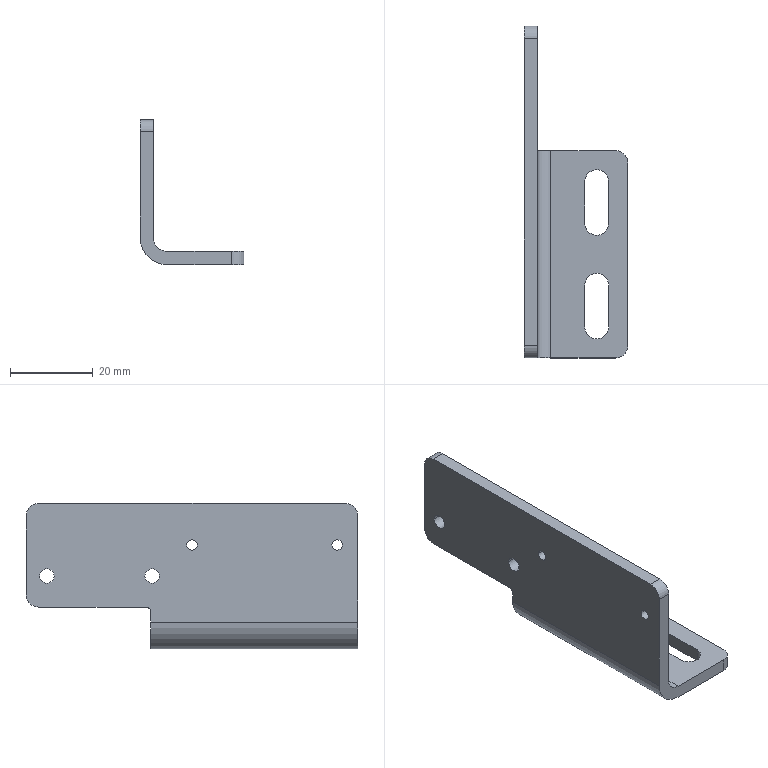Part | STEP file | J014-EBZ05-06-06-Part-1 | 1 solid | 34 faces | box 25 x 80 x 35 mm | volume 10495 mm3 | cylinder 20 | plane 14 | commonest cylinder face diameters 6 x5 2.5 x4 3.5 x4 5.8 x4 2 x1 6.4 x1
STEP:
#1=CARTESIAN_POINT('',(0.,3.75,25.));
#2=VERTEX_POINT('',#1);
#3=CARTESIAN_POINT('',(0.,6.25,25.));
#4=VERTEX_POINT('',#3);
#5=CARTESIAN_POINT('',(0.,5.,25.));
#6=DIRECTION('',(1.,0.,0.));
#7=DIRECTION('',(0.,1.,0.));
#8=AXIS2_PLACEMENT_3D('',#5,#6,#7);
#9=CIRCLE('',#8,1.25);
#10=EDGE_CURVE('',#2,#4,#9,.T.);
#11=ORIENTED_EDGE('',*,*,#10,.F.);
#12=CARTESIAN_POINT('',(3.2,3.75,25.));
#13=VERTEX_POINT('',#12);
#14=CARTESIAN_POINT('',(0.,3.75,25.));
#15=DIRECTION('',(1.,0.,0.));
#16=VECTOR('',#15,1000.);
#17=LINE('',#14,#16);
#18=EDGE_CURVE('',#2,#13,#17,.T.);
#19=ORIENTED_EDGE('',*,*,#18,.T.);
#20=CARTESIAN_POINT('',(3.2,6.25,25.));
#21=VERTEX_POINT('',#20);
#22=CARTESIAN_POINT('',(3.2,5.,25.));
#23=DIRECTION('',(-1.,0.,0.));
#24=DIRECTION('',(0.,-1.,0.));
#25=AXIS2_PLACEMENT_3D('',#22,#23,#24);
#26=CIRCLE('',#25,1.25);
#27=EDGE_CURVE('',#21,#13,#26,.T.);
#28=ORIENTED_EDGE('',*,*,#27,.F.);
#29=CARTESIAN_POINT('',(0.,6.25,25.));
#30=DIRECTION('',(1.,0.,0.));
#31=VECTOR('',#30,1000.);
#32=LINE('',#29,#31);
#33=EDGE_CURVE('',#4,#21,#32,.T.);
#34=ORIENTED_EDGE('',*,*,#33,.F.);
#35=EDGE_LOOP('',(#11,#19,#28,#34));
#36=FACE_OUTER_BOUND('',#35,.T.);
#37=CARTESIAN_POINT('',(0.,5.,25.));
#38=DIRECTION('',(1.,0.,0.));
#39=DIRECTION('',(0.,1.,0.));
#40=AXIS2_PLACEMENT_3D('',#37,#38,#39);
#41=CYLINDRICAL_SURFACE('',#40,1.25);
#42=ADVANCED_FACE('',(#36),#41,.F.);
#43=CARTESIAN_POINT('',(0.,38.75,25.));
#44=VERTEX_POINT('',#43);
#45=CARTESIAN_POINT('',(0.,41.25,25.));
#46=VERTEX_POINT('',#45);
#47=CARTESIAN_POINT('',(0.,40.,25.));
#48=DIRECTION('',(1.,0.,0.));
#49=DIRECTION('',(0.,1.,0.));
#50=AXIS2_PLACEMENT_3D('',#47,#48,#49);
#51=CIRCLE('',#50,1.25);
#52=EDGE_CURVE('',#44,#46,#51,.T.);
#53=ORIENTED_EDGE('',*,*,#52,.F.);
#54=CARTESIAN_POINT('',(3.2,38.75,25.));
#55=VERTEX_POINT('',#54);
#56=CARTESIAN_POINT('',(0.,38.75,25.));
#57=DIRECTION('',(1.,0.,0.));
#58=VECTOR('',#57,1000.);
#59=LINE('',#56,#58);
#60=EDGE_CURVE('',#44,#55,#59,.T.);
#61=ORIENTED_EDGE('',*,*,#60,.T.);
#62=CARTESIAN_POINT('',(3.2,41.25,25.));
#63=VERTEX_POINT('',#62);
#64=CARTESIAN_POINT('',(3.2,40.,25.));
#65=DIRECTION('',(-1.,0.,0.));
#66=DIRECTION('',(0.,-1.,0.));
#67=AXIS2_PLACEMENT_3D('',#64,#65,#66);
#68=CIRCLE('',#67,1.25);
#69=EDGE_CURVE('',#63,#55,#68,.T.);
#70=ORIENTED_EDGE('',*,*,#69,.F.);
#71=CARTESIAN_POINT('',(0.,41.25,25.));
#72=DIRECTION('',(1.,0.,0.));
#73=VECTOR('',#72,1000.);
#74=LINE('',#71,#73);
#75=EDGE_CURVE('',#46,#63,#74,.T.);
#76=ORIENTED_EDGE('',*,*,#75,.F.);
#77=EDGE_LOOP('',(#53,#61,#70,#76));
#78=FACE_OUTER_BOUND('',#77,.T.);
#79=CARTESIAN_POINT('',(0.,40.,25.));
#80=DIRECTION('',(1.,0.,0.));
#81=DIRECTION('',(0.,1.,0.));
#82=AXIS2_PLACEMENT_3D('',#79,#80,#81);
#83=CYLINDRICAL_SURFACE('',#82,1.25);
#84=ADVANCED_FACE('',(#78),#83,.F.);
#85=CARTESIAN_POINT('',(3.2,51.35,17.5));
#86=VERTEX_POINT('',#85);
#87=CARTESIAN_POINT('',(3.2,47.85,17.5));
#88=VERTEX_POINT('',#87);
#89=CARTESIAN_POINT('',(3.2,49.6,17.5));
#90=DIRECTION('',(-1.,0.,0.));
#91=DIRECTION('',(0.,-1.,0.));
#92=AXIS2_PLACEMENT_3D('',#89,#90,#91);
#93=CIRCLE('',#92,1.75);
#94=EDGE_CURVE('',#86,#88,#93,.T.);
#95=ORIENTED_EDGE('',*,*,#94,.F.);
#96=CARTESIAN_POINT('',(0.,51.35,17.5));
#97=VERTEX_POINT('',#96);
#98=CARTESIAN_POINT('',(3.2,51.35,17.5));
#99=DIRECTION('',(-1.,0.,0.));
#100=VECTOR('',#99,1000.);
#101=LINE('',#98,#100);
#102=EDGE_CURVE('',#86,#97,#101,.T.);
#103=ORIENTED_EDGE('',*,*,#102,.T.);
#104=CARTESIAN_POINT('',(0.,47.85,17.5));
#105=VERTEX_POINT('',#104);
#106=CARTESIAN_POINT('',(0.,49.6,17.5));
#107=DIRECTION('',(1.,0.,0.));
#108=DIRECTION('',(0.,1.,0.));
#109=AXIS2_PLACEMENT_3D('',#106,#107,#108);
#110=CIRCLE('',#109,1.75);
#111=EDGE_CURVE('',#105,#97,#110,.T.);
#112=ORIENTED_EDGE('',*,*,#111,.F.);
#113=CARTESIAN_POINT('',(3.2,47.85,17.5));
#114=DIRECTION('',(-1.,0.,0.));
#115=VECTOR('',#114,1000.);
#116=LINE('',#113,#115);
#117=EDGE_CURVE('',#88,#105,#116,.T.);
#118=ORIENTED_EDGE('',*,*,#117,.F.);
#119=EDGE_LOOP('',(#95,#103,#112,#118));
#120=FACE_OUTER_BOUND('',#119,.T.);
#121=CARTESIAN_POINT('',(3.2,49.6,17.5));
#122=DIRECTION('',(-1.,0.,0.));
#123=DIRECTION('',(0.,-1.,0.));
#124=AXIS2_PLACEMENT_3D('',#121,#122,#123);
#125=CYLINDRICAL_SURFACE('',#124,1.75);
#126=ADVANCED_FACE('',(#120),#125,.F.);
#127=CARTESIAN_POINT('',(3.2,76.75,17.5));
#128=VERTEX_POINT('',#127);
#129=CARTESIAN_POINT('',(3.2,73.25,17.5));
#130=VERTEX_POINT('',#129);
#131=CARTESIAN_POINT('',(3.2,75.,17.5));
#132=DIRECTION('',(-1.,0.,0.));
#133=DIRECTION('',(0.,-1.,0.));
#134=AXIS2_PLACEMENT_3D('',#131,#132,#133);
#135=CIRCLE('',#134,1.75);
#136=EDGE_CURVE('',#128,#130,#135,.T.);
#137=ORIENTED_EDGE('',*,*,#136,.F.);
#138=CARTESIAN_POINT('',(0.,76.75,17.5));
#139=VERTEX_POINT('',#138);
#140=CARTESIAN_POINT('',(3.2,76.75,17.5));
#141=DIRECTION('',(-1.,0.,0.));
#142=VECTOR('',#141,1000.);
#143=LINE('',#140,#142);
#144=EDGE_CURVE('',#128,#139,#143,.T.);
#145=ORIENTED_EDGE('',*,*,#144,.T.);
#146=CARTESIAN_POINT('',(0.,73.25,17.5));
#147=VERTEX_POINT('',#146);
#148=CARTESIAN_POINT('',(0.,75.,17.5));
#149=DIRECTION('',(1.,0.,0.));
#150=DIRECTION('',(0.,1.,0.));
#151=AXIS2_PLACEMENT_3D('',#148,#149,#150);
#152=CIRCLE('',#151,1.75);
#153=EDGE_CURVE('',#147,#139,#152,.T.);
#154=ORIENTED_EDGE('',*,*,#153,.F.);
#155=CARTESIAN_POINT('',(3.2,73.25,17.5));
#156=DIRECTION('',(-1.,0.,0.));
#157=VECTOR('',#156,1000.);
#158=LINE('',#155,#157);
#159=EDGE_CURVE('',#130,#147,#158,.T.);
#160=ORIENTED_EDGE('',*,*,#159,.F.);
#161=EDGE_LOOP('',(#137,#145,#154,#160));
#162=FACE_OUTER_BOUND('',#161,.T.);
#163=CARTESIAN_POINT('',(3.2,75.,17.5));
#164=DIRECTION('',(-1.,0.,0.));
#165=DIRECTION('',(0.,-1.,0.));
#166=AXIS2_PLACEMENT_3D('',#163,#164,#165);
#167=CYLINDRICAL_SURFACE('',#166,1.75);
#168=ADVANCED_FACE('',(#162),#167,.F.);
#169=CARTESIAN_POINT('',(25.,47.,3.2));
#170=VERTEX_POINT('',#169);
#171=CARTESIAN_POINT('',(25.,3.,3.2));
#172=VERTEX_POINT('',#171);
#173=CARTESIAN_POINT('',(25.,25.,3.2));
#174=DIRECTION('',(0.,-1.,0.));
#175=VECTOR('',#174,1000.);
#176=LINE('',#173,#175);
#177=EDGE_CURVE('',#170,#172,#176,.T.);
#178=ORIENTED_EDGE('',*,*,#177,.F.);
#179=CARTESIAN_POINT('',(22.,50.,3.2));
#180=VERTEX_POINT('',#179);
#181=CARTESIAN_POINT('',(22.,47.,3.2));
#182=DIRECTION('',(0.,0.,1.));
#183=DIRECTION('',(1.,0.,0.));
#184=AXIS2_PLACEMENT_3D('',#181,#182,#183);
#185=CIRCLE('',#184,3.);
#186=EDGE_CURVE('',#170,#180,#185,.T.);
#187=ORIENTED_EDGE('',*,*,#186,.T.);
#188=CARTESIAN_POINT('',(6.4,50.,3.2));
#189=VERTEX_POINT('',#188);
#190=CARTESIAN_POINT('',(12.5,50.,3.2));
#191=DIRECTION('',(1.,0.,0.));
#192=VECTOR('',#191,1000.);
#193=LINE('',#190,#192);
#194=EDGE_CURVE('',#189,#180,#193,.T.);
#195=ORIENTED_EDGE('',*,*,#194,.F.);
#196=CARTESIAN_POINT('',(6.4,0.,3.2));
#197=VERTEX_POINT('',#196);
#198=CARTESIAN_POINT('',(6.4,0.,3.2));
#199=DIRECTION('',(0.,-1.,0.));
#200=VECTOR('',#199,1000.);
#201=LINE('',#198,#200);
#202=EDGE_CURVE('',#189,#197,#201,.T.);
#203=ORIENTED_EDGE('',*,*,#202,.T.);
#204=CARTESIAN_POINT('',(22.,0.,3.2));
#205=VERTEX_POINT('',#204);
#206=CARTESIAN_POINT('',(12.5,0.,3.2));
#207=DIRECTION('',(-1.,0.,0.));
#208=VECTOR('',#207,1000.);
#209=LINE('',#206,#208);
#210=EDGE_CURVE('',#205,#197,#209,.T.);
#211=ORIENTED_EDGE('',*,*,#210,.F.);
#212=CARTESIAN_POINT('',(22.,3.,3.2));
#213=DIRECTION('',(0.,0.,1.));
#214=DIRECTION('',(1.,0.,0.));
#215=AXIS2_PLACEMENT_3D('',#212,#213,#214);
#216=CIRCLE('',#215,3.);
#217=EDGE_CURVE('',#205,#172,#216,.T.);
#218=ORIENTED_EDGE('',*,*,#217,.T.);
#219=EDGE_LOOP('',(#178,#187,#195,#203,#211,#218));
#220=FACE_OUTER_BOUND('',#219,.T.);
#221=CARTESIAN_POINT('',(14.6,7.5,3.2));
#222=VERTEX_POINT('',#221);
#223=CARTESIAN_POINT('',(14.6,17.5,3.2));
#224=VERTEX_POINT('',#223);
#225=CARTESIAN_POINT('',(14.6,12.5,3.2));
#226=DIRECTION('',(0.,1.,0.));
#227=VECTOR('',#226,1000.);
#228=LINE('',#225,#227);
#229=EDGE_CURVE('',#222,#224,#228,.T.);
#230=ORIENTED_EDGE('',*,*,#229,.T.);
#231=CARTESIAN_POINT('',(20.4,17.5,3.2));
#232=VERTEX_POINT('',#231);
#233=CARTESIAN_POINT('',(17.5,17.5,3.2));
#234=DIRECTION('',(0.,0.,-1.));
#235=DIRECTION('',(-1.,0.,0.));
#236=AXIS2_PLACEMENT_3D('',#233,#234,#235);
#237=CIRCLE('',#236,2.9);
#238=EDGE_CURVE('',#224,#232,#237,.T.);
#239=ORIENTED_EDGE('',*,*,#238,.T.);
#240=CARTESIAN_POINT('',(20.4,7.5,3.2));
#241=VERTEX_POINT('',#240);
#242=CARTESIAN_POINT('',(20.4,12.5,3.2));
#243=DIRECTION('',(0.,-1.,0.));
#244=VECTOR('',#243,1000.);
#245=LINE('',#242,#244);
#246=EDGE_CURVE('',#232,#241,#245,.T.);
#247=ORIENTED_EDGE('',*,*,#246,.T.);
#248=CARTESIAN_POINT('',(17.5,7.5,3.2));
#249=DIRECTION('',(0.,0.,-1.));
#250=DIRECTION('',(-1.,0.,0.));
#251=AXIS2_PLACEMENT_3D('',#248,#249,#250);
#252=CIRCLE('',#251,2.9);
#253=EDGE_CURVE('',#241,#222,#252,.T.);
#254=ORIENTED_EDGE('',*,*,#253,.T.);
#255=EDGE_LOOP('',(#230,#239,#247,#254));
#256=FACE_BOUND('',#255,.T.);
#257=CARTESIAN_POINT('',(14.6,32.5,3.2));
#258=VERTEX_POINT('',#257);
#259=CARTESIAN_POINT('',(14.6,42.5,3.2));
#260=VERTEX_POINT('',#259);
#261=CARTESIAN_POINT('',(14.6,37.5,3.2));
#262=DIRECTION('',(0.,1.,0.));
#263=VECTOR('',#262,1000.);
#264=LINE('',#261,#263);
#265=EDGE_CURVE('',#258,#260,#264,.T.);
#266=ORIENTED_EDGE('',*,*,#265,.T.);
#267=CARTESIAN_POINT('',(20.4,42.5,3.2));
#268=VERTEX_POINT('',#267);
#269=CARTESIAN_POINT('',(17.5,42.5,3.2));
#270=DIRECTION('',(0.,0.,-1.));
#271=DIRECTION('',(-1.,0.,0.));
#272=AXIS2_PLACEMENT_3D('',#269,#270,#271);
#273=CIRCLE('',#272,2.9);
#274=EDGE_CURVE('',#260,#268,#273,.T.);
#275=ORIENTED_EDGE('',*,*,#274,.T.);
#276=CARTESIAN_POINT('',(20.4,32.5,3.2));
#277=VERTEX_POINT('',#276);
#278=CARTESIAN_POINT('',(20.4,37.5,3.2));
#279=DIRECTION('',(0.,-1.,0.));
#280=VECTOR('',#279,1000.);
#281=LINE('',#278,#280);
#282=EDGE_CURVE('',#268,#277,#281,.T.);
#283=ORIENTED_EDGE('',*,*,#282,.T.);
#284=CARTESIAN_POINT('',(17.5,32.5,3.2));
#285=DIRECTION('',(0.,0.,-1.));
#286=DIRECTION('',(-1.,0.,0.));
#287=AXIS2_PLACEMENT_3D('',#284,#285,#286);
#288=CIRCLE('',#287,2.9);
#289=EDGE_CURVE('',#277,#258,#288,.T.);
#290=ORIENTED_EDGE('',*,*,#289,.T.);
#291=EDGE_LOOP('',(#266,#275,#283,#290));
#292=FACE_BOUND('',#291,.T.);
#293=CARTESIAN_POINT('',(12.5,25.,3.2));
#294=DIRECTION('',(0.,0.,1.));
#295=DIRECTION('',(1.,0.,0.));
#296=AXIS2_PLACEMENT_3D('',#293,#294,#295);
#297=PLANE('',#296);
#298=ADVANCED_FACE('',(#220,#256,#292),#297,.T.);
#299=CARTESIAN_POINT('',(22.,50.,0.));
#300=VERTEX_POINT('',#299);
#301=CARTESIAN_POINT('',(6.4,50.,0.));
#302=VERTEX_POINT('',#301);
#303=CARTESIAN_POINT('',(12.5,50.,0.));
#304=DIRECTION('',(-1.,0.,0.));
#305=VECTOR('',#304,1000.);
#306=LINE('',#303,#305);
#307=EDGE_CURVE('',#300,#302,#306,.T.);
#308=ORIENTED_EDGE('',*,*,#307,.F.);
#309=CARTESIAN_POINT('',(25.,47.,0.));
#310=VERTEX_POINT('',#309);
#311=CARTESIAN_POINT('',(22.,47.,0.));
#312=DIRECTION('',(0.,0.,-1.));
#313=DIRECTION('',(-1.,0.,0.));
#314=AXIS2_PLACEMENT_3D('',#311,#312,#313);
#315=CIRCLE('',#314,3.);
#316=EDGE_CURVE('',#300,#310,#315,.T.);
#317=ORIENTED_EDGE('',*,*,#316,.T.);
#318=CARTESIAN_POINT('',(25.,3.,0.));
#319=VERTEX_POINT('',#318);
#320=CARTESIAN_POINT('',(25.,25.,0.));
#321=DIRECTION('',(0.,1.,0.));
#322=VECTOR('',#321,1000.);
#323=LINE('',#320,#322);
#324=EDGE_CURVE('',#319,#310,#323,.T.);
#325=ORIENTED_EDGE('',*,*,#324,.F.);
#326=CARTESIAN_POINT('',(22.,0.,0.));
#327=VERTEX_POINT('',#326);
#328=CARTESIAN_POINT('',(22.,3.,0.));
#329=DIRECTION('',(0.,0.,-1.));
#330=DIRECTION('',(-1.,0.,0.));
#331=AXIS2_PLACEMENT_3D('',#328,#329,#330);
#332=CIRCLE('',#331,3.);
#333=EDGE_CURVE('',#319,#327,#332,.T.);
#334=ORIENTED_EDGE('',*,*,#333,.T.);
#335=CARTESIAN_POINT('',(6.4,0.,0.));
#336=VERTEX_POINT('',#335);
#337=CARTESIAN_POINT('',(12.5,0.,0.));
#338=DIRECTION('',(1.,0.,0.));
#339=VECTOR('',#338,1000.);
#340=LINE('',#337,#339);
#341=EDGE_CURVE('',#336,#327,#340,.T.);
#342=ORIENTED_EDGE('',*,*,#341,.F.);
#343=CARTESIAN_POINT('',(6.4,25.,0.));
#344=DIRECTION('',(0.,1.,0.));
#345=VECTOR('',#344,1000.);
#346=LINE('',#343,#345);
#347=EDGE_CURVE('',#336,#302,#346,.T.);
#348=ORIENTED_EDGE('',*,*,#347,.T.);
#349=EDGE_LOOP('',(#308,#317,#325,#334,#342,#348));
#350=FACE_OUTER_BOUND('',#349,.T.);
#351=CARTESIAN_POINT('',(20.4,7.5,0.));
#352=VERTEX_POINT('',#351);
#353=CARTESIAN_POINT('',(20.4,17.5,0.));
#354=VERTEX_POINT('',#353);
#355=CARTESIAN_POINT('',(20.4,12.5,0.));
#356=DIRECTION('',(0.,1.,0.));
#357=VECTOR('',#356,1000.);
#358=LINE('',#355,#357);
#359=EDGE_CURVE('',#352,#354,#358,.T.);
#360=ORIENTED_EDGE('',*,*,#359,.T.);
#361=CARTESIAN_POINT('',(14.6,17.5,0.));
#362=VERTEX_POINT('',#361);
#363=CARTESIAN_POINT('',(17.5,17.5,0.));
#364=DIRECTION('',(0.,0.,1.));
#365=DIRECTION('',(1.,0.,0.));
#366=AXIS2_PLACEMENT_3D('',#363,#364,#365);
#367=CIRCLE('',#366,2.9);
#368=EDGE_CURVE('',#354,#362,#367,.T.);
#369=ORIENTED_EDGE('',*,*,#368,.T.);
#370=CARTESIAN_POINT('',(14.6,7.5,0.));
#371=VERTEX_POINT('',#370);
#372=CARTESIAN_POINT('',(14.6,12.5,0.));
#373=DIRECTION('',(0.,-1.,0.));
#374=VECTOR('',#373,1000.);
#375=LINE('',#372,#374);
#376=EDGE_CURVE('',#362,#371,#375,.T.);
#377=ORIENTED_EDGE('',*,*,#376,.T.);
#378=CARTESIAN_POINT('',(17.5,7.5,0.));
#379=DIRECTION('',(0.,0.,1.));
#380=DIRECTION('',(1.,0.,0.));
#381=AXIS2_PLACEMENT_3D('',#378,#379,#380);
#382=CIRCLE('',#381,2.9);
#383=EDGE_CURVE('',#371,#352,#382,.T.);
#384=ORIENTED_EDGE('',*,*,#383,.T.);
#385=EDGE_LOOP('',(#360,#369,#377,#384));
#386=FACE_BOUND('',#385,.T.);
#387=CARTESIAN_POINT('',(20.4,32.5,0.));
#388=VERTEX_POINT('',#387);
#389=CARTESIAN_POINT('',(20.4,42.5,0.));
#390=VERTEX_POINT('',#389);
#391=CARTESIAN_POINT('',(20.4,37.5,0.));
#392=DIRECTION('',(0.,1.,0.));
#393=VECTOR('',#392,1000.);
#394=LINE('',#391,#393);
#395=EDGE_CURVE('',#388,#390,#394,.T.);
#396=ORIENTED_EDGE('',*,*,#395,.T.);
#397=CARTESIAN_POINT('',(14.6,42.5,0.));
#398=VERTEX_POINT('',#397);
#399=CARTESIAN_POINT('',(17.5,42.5,0.));
#400=DIRECTION('',(0.,0.,1.));
#401=DIRECTION('',(1.,0.,0.));
#402=AXIS2_PLACEMENT_3D('',#399,#400,#401);
#403=CIRCLE('',#402,2.9);
#404=EDGE_CURVE('',#390,#398,#403,.T.);
#405=ORIENTED_EDGE('',*,*,#404,.T.);
#406=CARTESIAN_POINT('',(14.6,32.5,0.));
#407=VERTEX_POINT('',#406);
#408=CARTESIAN_POINT('',(14.6,37.5,0.));
#409=DIRECTION('',(0.,-1.,0.));
#410=VECTOR('',#409,1000.);
#411=LINE('',#408,#410);
#412=EDGE_CURVE('',#398,#407,#411,.T.);
#413=ORIENTED_EDGE('',*,*,#412,.T.);
#414=CARTESIAN_POINT('',(17.5,32.5,0.));
#415=DIRECTION('',(0.,0.,1.));
#416=DIRECTION('',(1.,0.,0.));
#417=AXIS2_PLACEMENT_3D('',#414,#415,#416);
#418=CIRCLE('',#417,2.9);
#419=EDGE_CURVE('',#407,#388,#418,.T.);
#420=ORIENTED_EDGE('',*,*,#419,.T.);
#421=EDGE_LOOP('',(#396,#405,#413,#420));
#422=FACE_BOUND('',#421,.T.);
#423=CARTESIAN_POINT('',(12.5,25.,0.));
#424=DIRECTION('',(0.,0.,-1.));
#425=DIRECTION('',(-1.,0.,0.));
#426=AXIS2_PLACEMENT_3D('',#423,#424,#425);
#427=PLANE('',#426);
#428=ADVANCED_FACE('',(#350,#386,#422),#427,.T.);
#429=CARTESIAN_POINT('',(3.2,0.,6.4));
#430=VERTEX_POINT('',#429);
#431=CARTESIAN_POINT('',(3.2,0.,32.));
#432=VERTEX_POINT('',#431);
#433=CARTESIAN_POINT('',(3.2,0.,5.));
#434=DIRECTION('',(0.,0.,1.));
#435=VECTOR('',#434,1000.);
#436=LINE('',#433,#435);
#437=EDGE_CURVE('',#430,#432,#436,.T.);
#438=ORIENTED_EDGE('',*,*,#437,.T.);
#439=CARTESIAN_POINT('',(0.,0.,32.));
#440=VERTEX_POINT('',#439);
#441=CARTESIAN_POINT('',(12.5,0.,32.));
#442=DIRECTION('',(-1.,0.,0.));
#443=VECTOR('',#442,1000.);
#444=LINE('',#441,#443);
#445=EDGE_CURVE('',#432,#440,#444,.T.);
#446=ORIENTED_EDGE('',*,*,#445,.T.);
#447=CARTESIAN_POINT('',(0.,0.,6.4));
#448=VERTEX_POINT('',#447);
#449=CARTESIAN_POINT('',(0.,0.,0.));
#450=DIRECTION('',(0.,0.,1.));
#451=VECTOR('',#450,1000.);
#452=LINE('',#449,#451);
#453=EDGE_CURVE('',#448,#440,#452,.T.);
#454=ORIENTED_EDGE('',*,*,#453,.F.);
#455=CARTESIAN_POINT('',(6.4,0.,6.4));
#456=DIRECTION('',(0.,-1.,0.));
#457=DIRECTION('',(0.,0.,-1.));
#458=AXIS2_PLACEMENT_3D('',#455,#456,#457);
#459=CIRCLE('',#458,6.4);
#460=EDGE_CURVE('',#448,#336,#459,.T.);
#461=ORIENTED_EDGE('',*,*,#460,.T.);
#462=ORIENTED_EDGE('',*,*,#341,.T.);
#463=CARTESIAN_POINT('',(22.,0.,0.));
#464=DIRECTION('',(0.,0.,1.));
#465=VECTOR('',#464,1000.);
#466=LINE('',#463,#465);
#467=EDGE_CURVE('',#327,#205,#466,.T.);
#468=ORIENTED_EDGE('',*,*,#467,.T.);
#469=ORIENTED_EDGE('',*,*,#210,.T.);
#470=CARTESIAN_POINT('',(6.4,0.,6.4));
#471=DIRECTION('',(0.,1.,0.));
#472=DIRECTION('',(0.,0.,-1.));
#473=AXIS2_PLACEMENT_3D('',#470,#471,#472);
#474=CIRCLE('',#473,3.2);
#475=EDGE_CURVE('',#197,#430,#474,.T.);
#476=ORIENTED_EDGE('',*,*,#475,.T.);
#477=EDGE_LOOP('',(#438,#446,#454,#461,#462,#468,#469,#476));
#478=FACE_OUTER_BOUND('',#477,.T.);
#479=CARTESIAN_POINT('',(12.5,0.,0.));
#480=DIRECTION('',(0.,-1.,0.));
#481=DIRECTION('',(0.,0.,-1.));
#482=AXIS2_PLACEMENT_3D('',#479,#480,#481);
#483=PLANE('',#482);
#484=ADVANCED_FACE('',(#478),#483,.T.);
#485=CARTESIAN_POINT('',(0.,5.,25.));
#486=DIRECTION('',(1.,0.,0.));
#487=DIRECTION('',(0.,1.,0.));
#488=AXIS2_PLACEMENT_3D('',#485,#486,#487);
#489=CIRCLE('',#488,1.25);
#490=EDGE_CURVE('',#4,#2,#489,.T.);
#491=ORIENTED_EDGE('',*,*,#490,.T.);
#492=ORIENTED_EDGE('',*,*,#10,.T.);
#493=EDGE_LOOP('',(#491,#492));
#494=FACE_BOUND('',#493,.T.);
#495=CARTESIAN_POINT('',(0.,40.,25.));
#496=DIRECTION('',(1.,0.,0.));
#497=DIRECTION('',(0.,1.,0.));
#498=AXIS2_PLACEMENT_3D('',#495,#496,#497);
#499=CIRCLE('',#498,1.25);
#500=EDGE_CURVE('',#46,#44,#499,.T.);
#501=ORIENTED_EDGE('',*,*,#500,.T.);
#502=ORIENTED_EDGE('',*,*,#52,.T.);
#503=EDGE_LOOP('',(#501,#502));
#504=FACE_BOUND('',#503,.T.);
#505=ORIENTED_EDGE('',*,*,#111,.T.);
#506=CARTESIAN_POINT('',(0.,49.6,17.5));
#507=DIRECTION('',(1.,0.,0.));
#508=DIRECTION('',(0.,1.,0.));
#509=AXIS2_PLACEMENT_3D('',#506,#507,#508);
#510=CIRCLE('',#509,1.75);
#511=EDGE_CURVE('',#97,#105,#510,.T.);
#512=ORIENTED_EDGE('',*,*,#511,.T.);
#513=EDGE_LOOP('',(#505,#512));
#514=FACE_BOUND('',#513,.T.);
#515=ORIENTED_EDGE('',*,*,#153,.T.);
#516=CARTESIAN_POINT('',(0.,75.,17.5));
#517=DIRECTION('',(1.,0.,0.));
#518=DIRECTION('',(0.,1.,0.));
#519=AXIS2_PLACEMENT_3D('',#516,#517,#518);
#520=CIRCLE('',#519,1.75);
#521=EDGE_CURVE('',#139,#147,#520,.T.);
#522=ORIENTED_EDGE('',*,*,#521,.T.);
#523=EDGE_LOOP('',(#515,#522));
#524=FACE_BOUND('',#523,.T.);
#525=ORIENTED_EDGE('',*,*,#453,.T.);
#526=CARTESIAN_POINT('',(0.,3.,35.));
#527=VERTEX_POINT('',#526);
#528=CARTESIAN_POINT('',(0.,3.,32.));
#529=DIRECTION('',(-1.,0.,0.));
#530=DIRECTION('',(0.,0.,1.));
#531=AXIS2_PLACEMENT_3D('',#528,#529,#530);
#532=CIRCLE('',#531,3.);
#533=EDGE_CURVE('',#440,#527,#532,.T.);
#534=ORIENTED_EDGE('',*,*,#533,.T.);
#535=CARTESIAN_POINT('',(0.,77.,35.));
#536=VERTEX_POINT('',#535);
#537=CARTESIAN_POINT('',(0.,40.,35.));
#538=DIRECTION('',(0.,-1.,0.));
#539=VECTOR('',#538,1000.);
#540=LINE('',#537,#539);
#541=EDGE_CURVE('',#536,#527,#540,.T.);
#542=ORIENTED_EDGE('',*,*,#541,.F.);
#543=CARTESIAN_POINT('',(0.,80.,32.));
#544=VERTEX_POINT('',#543);
#545=CARTESIAN_POINT('',(0.,77.,32.));
#546=DIRECTION('',(-1.,0.,0.));
#547=DIRECTION('',(0.,0.,1.));
#548=AXIS2_PLACEMENT_3D('',#545,#546,#547);
#549=CIRCLE('',#548,3.);
#550=EDGE_CURVE('',#536,#544,#549,.T.);
#551=ORIENTED_EDGE('',*,*,#550,.T.);
#552=CARTESIAN_POINT('',(0.,80.,13.));
#553=VERTEX_POINT('',#552);
#554=CARTESIAN_POINT('',(0.,80.,22.5));
#555=DIRECTION('',(0.,0.,1.));
#556=VECTOR('',#555,1000.);
#557=LINE('',#554,#556);
#558=EDGE_CURVE('',#553,#544,#557,.T.);
#559=ORIENTED_EDGE('',*,*,#558,.F.);
#560=CARTESIAN_POINT('',(0.,77.,10.));
#561=VERTEX_POINT('',#560);
#562=CARTESIAN_POINT('',(0.,77.,13.));
#563=DIRECTION('',(-1.,0.,0.));
#564=DIRECTION('',(0.,0.,1.));
#565=AXIS2_PLACEMENT_3D('',#562,#563,#564);
#566=CIRCLE('',#565,3.);
#567=EDGE_CURVE('',#553,#561,#566,.T.);
#568=ORIENTED_EDGE('',*,*,#567,.T.);
#569=CARTESIAN_POINT('',(0.,51.,10.));
#570=VERTEX_POINT('',#569);
#571=CARTESIAN_POINT('',(0.,40.,10.));
#572=DIRECTION('',(0.,1.,0.));
#573=VECTOR('',#572,1000.);
#574=LINE('',#571,#573);
#575=EDGE_CURVE('',#570,#561,#574,.T.);
#576=ORIENTED_EDGE('',*,*,#575,.F.);
#577=CARTESIAN_POINT('',(0.,50.,9.));
#578=VERTEX_POINT('',#577);
#579=CARTESIAN_POINT('',(0.,51.,9.));
#580=DIRECTION('',(1.,0.,0.));
#581=DIRECTION('',(0.,0.,1.));
#582=AXIS2_PLACEMENT_3D('',#579,#580,#581);
#583=CIRCLE('',#582,1.);
#584=EDGE_CURVE('',#570,#578,#583,.T.);
#585=ORIENTED_EDGE('',*,*,#584,.T.);
#586=CARTESIAN_POINT('',(0.,50.,6.4));
#587=VERTEX_POINT('',#586);
#588=CARTESIAN_POINT('',(0.,50.,0.));
#589=DIRECTION('',(0.,0.,1.));
#590=VECTOR('',#589,1000.);
#591=LINE('',#588,#590);
#592=EDGE_CURVE('',#587,#578,#591,.T.);
#593=ORIENTED_EDGE('',*,*,#592,.F.);
#594=CARTESIAN_POINT('',(0.,25.,6.4));
#595=DIRECTION('',(0.,-1.,0.));
#596=VECTOR('',#595,1000.);
#597=LINE('',#594,#596);
#598=EDGE_CURVE('',#587,#448,#597,.T.);
#599=ORIENTED_EDGE('',*,*,#598,.T.);
#600=EDGE_LOOP('',(#525,#534,#542,#551,#559,#568,#576,#585,#593,#599));
#601=FACE_OUTER_BOUND('',#600,.T.);
#602=CARTESIAN_POINT('',(0.,25.,0.));
#603=DIRECTION('',(-1.,0.,0.));
#604=DIRECTION('',(0.,0.,1.));
#605=AXIS2_PLACEMENT_3D('',#602,#603,#604);
#606=PLANE('',#605);
#607=ADVANCED_FACE('',(#494,#504,#514,#524,#601),#606,.T.);
#608=ORIENTED_EDGE('',*,*,#592,.T.);
#609=CARTESIAN_POINT('',(3.2,50.,9.));
#610=VERTEX_POINT('',#609);
#611=CARTESIAN_POINT('',(3.2,50.,9.));
#612=DIRECTION('',(1.,0.,0.));
#613=VECTOR('',#612,1000.);
#614=LINE('',#611,#613);
#615=EDGE_CURVE('',#578,#610,#614,.T.);
#616=ORIENTED_EDGE('',*,*,#615,.T.);
#617=CARTESIAN_POINT('',(3.2,50.,6.4));
#618=VERTEX_POINT('',#617);
#619=CARTESIAN_POINT('',(3.2,50.,5.));
#620=DIRECTION('',(0.,0.,-1.));
#621=VECTOR('',#620,1000.);
#622=LINE('',#619,#621);
#623=EDGE_CURVE('',#610,#618,#622,.T.);
#624=ORIENTED_EDGE('',*,*,#623,.T.);
#625=CARTESIAN_POINT('',(6.4,50.,6.4));
#626=DIRECTION('',(0.,-1.,0.));
#627=DIRECTION('',(0.,0.,1.));
#628=AXIS2_PLACEMENT_3D('',#625,#626,#627);
#629=CIRCLE('',#628,3.2);
#630=EDGE_CURVE('',#618,#189,#629,.T.);
#631=ORIENTED_EDGE('',*,*,#630,.T.);
#632=ORIENTED_EDGE('',*,*,#194,.T.);
#633=CARTESIAN_POINT('',(22.,50.,0.));
#634=DIRECTION('',(0.,0.,-1.));
#635=VECTOR('',#634,1000.);
#636=LINE('',#633,#635);
#637=EDGE_CURVE('',#180,#300,#636,.T.);
#638=ORIENTED_EDGE('',*,*,#637,.T.);
#639=ORIENTED_EDGE('',*,*,#307,.T.);
#640=CARTESIAN_POINT('',(6.4,50.,6.4));
#641=DIRECTION('',(0.,1.,0.));
#642=DIRECTION('',(0.,0.,1.));
#643=AXIS2_PLACEMENT_3D('',#640,#641,#642);
#644=CIRCLE('',#643,6.4);
#645=EDGE_CURVE('',#302,#587,#644,.T.);
#646=ORIENTED_EDGE('',*,*,#645,.T.);
#647=EDGE_LOOP('',(#608,#616,#624,#631,#632,#638,#639,#646));
#648=FACE_OUTER_BOUND('',#647,.T.);
#649=CARTESIAN_POINT('',(12.5,50.,0.));
#650=DIRECTION('',(0.,1.,0.));
#651=DIRECTION('',(0.,0.,1.));
#652=AXIS2_PLACEMENT_3D('',#649,#650,#651);
#653=PLANE('',#652);
#654=ADVANCED_FACE('',(#648),#653,.T.);
#655=ORIENTED_EDGE('',*,*,#324,.T.);
#656=CARTESIAN_POINT('',(25.,47.,0.));
#657=DIRECTION('',(0.,0.,1.));
#658=VECTOR('',#657,1000.);
#659=LINE('',#656,#658);
#660=EDGE_CURVE('',#310,#170,#659,.T.);
#661=ORIENTED_EDGE('',*,*,#660,.T.);
#662=ORIENTED_EDGE('',*,*,#177,.T.);
#663=CARTESIAN_POINT('',(25.,3.,0.));
#664=DIRECTION('',(0.,0.,-1.));
#665=VECTOR('',#664,1000.);
#666=LINE('',#663,#665);
#667=EDGE_CURVE('',#172,#319,#666,.T.);
#668=ORIENTED_EDGE('',*,*,#667,.T.);
#669=EDGE_LOOP('',(#655,#661,#662,#668));
#670=FACE_OUTER_BOUND('',#669,.T.);
#671=CARTESIAN_POINT('',(25.,25.,0.));
#672=DIRECTION('',(1.,0.,0.));
#673=DIRECTION('',(0.,0.,-1.));
#674=AXIS2_PLACEMENT_3D('',#671,#672,#673);
#675=PLANE('',#674);
#676=ADVANCED_FACE('',(#670),#675,.T.);
#677=ORIENTED_EDGE('',*,*,#27,.T.);
#678=CARTESIAN_POINT('',(3.2,5.,25.));
#679=DIRECTION('',(-1.,0.,0.));
#680=DIRECTION('',(0.,-1.,0.));
#681=AXIS2_PLACEMENT_3D('',#678,#679,#680);
#682=CIRCLE('',#681,1.25);
#683=EDGE_CURVE('',#13,#21,#682,.T.);
#684=ORIENTED_EDGE('',*,*,#683,.T.);
#685=EDGE_LOOP('',(#677,#684));
#686=FACE_BOUND('',#685,.T.);
#687=ORIENTED_EDGE('',*,*,#69,.T.);
#688=CARTESIAN_POINT('',(3.2,40.,25.));
#689=DIRECTION('',(-1.,0.,0.));
#690=DIRECTION('',(0.,-1.,0.));
#691=AXIS2_PLACEMENT_3D('',#688,#689,#690);
#692=CIRCLE('',#691,1.25);
#693=EDGE_CURVE('',#55,#63,#692,.T.);
#694=ORIENTED_EDGE('',*,*,#693,.T.);
#695=EDGE_LOOP('',(#687,#694));
#696=FACE_BOUND('',#695,.T.);
#697=CARTESIAN_POINT('',(3.2,49.6,17.5));
#698=DIRECTION('',(-1.,0.,0.));
#699=DIRECTION('',(0.,-1.,0.));
#700=AXIS2_PLACEMENT_3D('',#697,#698,#699);
#701=CIRCLE('',#700,1.75);
#702=EDGE_CURVE('',#88,#86,#701,.T.);
#703=ORIENTED_EDGE('',*,*,#702,.T.);
#704=ORIENTED_EDGE('',*,*,#94,.T.);
#705=EDGE_LOOP('',(#703,#704));
#706=FACE_BOUND('',#705,.T.);
#707=CARTESIAN_POINT('',(3.2,75.,17.5));
#708=DIRECTION('',(-1.,0.,0.));
#709=DIRECTION('',(0.,-1.,0.));
#710=AXIS2_PLACEMENT_3D('',#707,#708,#709);
#711=CIRCLE('',#710,1.75);
#712=EDGE_CURVE('',#130,#128,#711,.T.);
#713=ORIENTED_EDGE('',*,*,#712,.T.);
#714=ORIENTED_EDGE('',*,*,#136,.T.);
#715=EDGE_LOOP('',(#713,#714));
#716=FACE_BOUND('',#715,.T.);
#717=CARTESIAN_POINT('',(3.2,3.,35.));
#718=VERTEX_POINT('',#717);
#719=CARTESIAN_POINT('',(3.2,77.,35.));
#720=VERTEX_POINT('',#719);
#721=CARTESIAN_POINT('',(3.2,40.,35.));
#722=DIRECTION('',(0.,1.,0.));
#723=VECTOR('',#722,1000.);
#724=LINE('',#721,#723);
#725=EDGE_CURVE('',#718,#720,#724,.T.);
#726=ORIENTED_EDGE('',*,*,#725,.F.);
#727=CARTESIAN_POINT('',(3.2,3.,32.));
#728=DIRECTION('',(1.,0.,0.));
#729=DIRECTION('',(0.,1.,0.));
#730=AXIS2_PLACEMENT_3D('',#727,#728,#729);
#731=CIRCLE('',#730,3.);
#732=EDGE_CURVE('',#718,#432,#731,.T.);
#733=ORIENTED_EDGE('',*,*,#732,.T.);
#734=ORIENTED_EDGE('',*,*,#437,.F.);
#735=CARTESIAN_POINT('',(3.2,50.,6.4));
#736=DIRECTION('',(0.,1.,0.));
#737=VECTOR('',#736,1000.);
#738=LINE('',#735,#737);
#739=EDGE_CURVE('',#430,#618,#738,.T.);
#740=ORIENTED_EDGE('',*,*,#739,.T.);
#741=ORIENTED_EDGE('',*,*,#623,.F.);
#742=CARTESIAN_POINT('',(3.2,51.,10.));
#743=VERTEX_POINT('',#742);
#744=CARTESIAN_POINT('',(3.2,51.,9.));
#745=DIRECTION('',(-1.,0.,0.));
#746=DIRECTION('',(0.,1.,0.));
#747=AXIS2_PLACEMENT_3D('',#744,#745,#746);
#748=CIRCLE('',#747,1.);
#749=EDGE_CURVE('',#610,#743,#748,.T.);
#750=ORIENTED_EDGE('',*,*,#749,.T.);
#751=CARTESIAN_POINT('',(3.2,77.,10.));
#752=VERTEX_POINT('',#751);
#753=CARTESIAN_POINT('',(3.2,40.,10.));
#754=DIRECTION('',(0.,-1.,0.));
#755=VECTOR('',#754,1000.);
#756=LINE('',#753,#755);
#757=EDGE_CURVE('',#752,#743,#756,.T.);
#758=ORIENTED_EDGE('',*,*,#757,.F.);
#759=CARTESIAN_POINT('',(3.2,80.,13.));
#760=VERTEX_POINT('',#759);
#761=CARTESIAN_POINT('',(3.2,77.,13.));
#762=DIRECTION('',(1.,0.,0.));
#763=DIRECTION('',(0.,1.,0.));
#764=AXIS2_PLACEMENT_3D('',#761,#762,#763);
#765=CIRCLE('',#764,3.);
#766=EDGE_CURVE('',#752,#760,#765,.T.);
#767=ORIENTED_EDGE('',*,*,#766,.T.);
#768=CARTESIAN_POINT('',(3.2,80.,32.));
#769=VERTEX_POINT('',#768);
#770=CARTESIAN_POINT('',(3.2,80.,22.5));
#771=DIRECTION('',(0.,0.,-1.));
#772=VECTOR('',#771,1000.);
#773=LINE('',#770,#772);
#774=EDGE_CURVE('',#769,#760,#773,.T.);
#775=ORIENTED_EDGE('',*,*,#774,.F.);
#776=CARTESIAN_POINT('',(3.2,77.,32.));
#777=DIRECTION('',(1.,0.,0.));
#778=DIRECTION('',(0.,1.,0.));
#779=AXIS2_PLACEMENT_3D('',#776,#777,#778);
#780=CIRCLE('',#779,3.);
#781=EDGE_CURVE('',#769,#720,#780,.T.);
#782=ORIENTED_EDGE('',*,*,#781,.T.);
#783=EDGE_LOOP('',(#726,#733,#734,#740,#741,#750,#758,#767,#775,#782));
#784=FACE_OUTER_BOUND('',#783,.T.);
#785=CARTESIAN_POINT('',(3.2,25.,5.));
#786=DIRECTION('',(1.,0.,0.));
#787=DIRECTION('',(0.,0.,-1.));
#788=AXIS2_PLACEMENT_3D('',#785,#786,#787);
#789=PLANE('',#788);
#790=ADVANCED_FACE('',(#686,#696,#706,#716,#784),#789,.T.);
#791=ORIENTED_EDGE('',*,*,#757,.T.);
#792=CARTESIAN_POINT('',(0.,51.,10.));
#793=DIRECTION('',(-1.,0.,0.));
#794=VECTOR('',#793,1000.);
#795=LINE('',#792,#794);
#796=EDGE_CURVE('',#743,#570,#795,.T.);
#797=ORIENTED_EDGE('',*,*,#796,.T.);
#798=ORIENTED_EDGE('',*,*,#575,.T.);
#799=CARTESIAN_POINT('',(3.2,77.,10.));
#800=DIRECTION('',(1.,0.,0.));
#801=VECTOR('',#800,1000.);
#802=LINE('',#799,#801);
#803=EDGE_CURVE('',#561,#752,#802,.T.);
#804=ORIENTED_EDGE('',*,*,#803,.T.);
#805=EDGE_LOOP('',(#791,#797,#798,#804));
#806=FACE_OUTER_BOUND('',#805,.T.);
#807=CARTESIAN_POINT('',(3.2,40.,10.));
#808=DIRECTION('',(0.,0.,-1.));
#809=DIRECTION('',(-1.,0.,0.));
#810=AXIS2_PLACEMENT_3D('',#807,#808,#809);
#811=PLANE('',#810);
#812=ADVANCED_FACE('',(#806),#811,.T.);
#813=ORIENTED_EDGE('',*,*,#558,.T.);
#814=CARTESIAN_POINT('',(3.2,80.,32.));
#815=DIRECTION('',(1.,0.,0.));
#816=VECTOR('',#815,1000.);
#817=LINE('',#814,#816);
#818=EDGE_CURVE('',#544,#769,#817,.T.);
#819=ORIENTED_EDGE('',*,*,#818,.T.);
#820=ORIENTED_EDGE('',*,*,#774,.T.);
#821=CARTESIAN_POINT('',(3.2,80.,13.));
#822=DIRECTION('',(-1.,0.,0.));
#823=VECTOR('',#822,1000.);
#824=LINE('',#821,#823);
#825=EDGE_CURVE('',#760,#553,#824,.T.);
#826=ORIENTED_EDGE('',*,*,#825,.T.);
#827=EDGE_LOOP('',(#813,#819,#820,#826));
#828=FACE_OUTER_BOUND('',#827,.T.);
#829=CARTESIAN_POINT('',(3.2,80.,22.5));
#830=DIRECTION('',(0.,1.,0.));
#831=DIRECTION('',(-1.,0.,0.));
#832=AXIS2_PLACEMENT_3D('',#829,#830,#831);
#833=PLANE('',#832);
#834=ADVANCED_FACE('',(#828),#833,.T.);
#835=ORIENTED_EDGE('',*,*,#541,.T.);
#836=CARTESIAN_POINT('',(3.2,3.,35.));
#837=DIRECTION('',(1.,0.,0.));
#838=VECTOR('',#837,1000.);
#839=LINE('',#836,#838);
#840=EDGE_CURVE('',#527,#718,#839,.T.);
#841=ORIENTED_EDGE('',*,*,#840,.T.);
#842=ORIENTED_EDGE('',*,*,#725,.T.);
#843=CARTESIAN_POINT('',(3.2,77.,35.));
#844=DIRECTION('',(-1.,0.,0.));
#845=VECTOR('',#844,1000.);
#846=LINE('',#843,#845);
#847=EDGE_CURVE('',#720,#536,#846,.T.);
#848=ORIENTED_EDGE('',*,*,#847,.T.);
#849=EDGE_LOOP('',(#835,#841,#842,#848));
#850=FACE_OUTER_BOUND('',#849,.T.);
#851=CARTESIAN_POINT('',(3.2,40.,35.));
#852=DIRECTION('',(0.,0.,1.));
#853=DIRECTION('',(1.,0.,0.));
#854=AXIS2_PLACEMENT_3D('',#851,#852,#853);
#855=PLANE('',#854);
#856=ADVANCED_FACE('',(#850),#855,.T.);
#857=CARTESIAN_POINT('',(14.6,7.5,0.));
#858=DIRECTION('',(0.,0.,1.));
#859=VECTOR('',#858,1000.);
#860=LINE('',#857,#859);
#861=EDGE_CURVE('',#371,#222,#860,.T.);
#862=ORIENTED_EDGE('',*,*,#861,.F.);
#863=ORIENTED_EDGE('',*,*,#376,.F.);
#864=CARTESIAN_POINT('',(14.6,17.5,0.));
#865=DIRECTION('',(0.,0.,1.));
#866=VECTOR('',#865,1000.);
#867=LINE('',#864,#866);
#868=EDGE_CURVE('',#362,#224,#867,.T.);
#869=ORIENTED_EDGE('',*,*,#868,.T.);
#870=ORIENTED_EDGE('',*,*,#229,.F.);
#871=EDGE_LOOP('',(#862,#863,#869,#870));
#872=FACE_OUTER_BOUND('',#871,.T.);
#873=CARTESIAN_POINT('',(14.6,12.5,0.));
#874=DIRECTION('',(-1.,0.,0.));
#875=DIRECTION('',(0.,0.,-1.));
#876=AXIS2_PLACEMENT_3D('',#873,#874,#875);
#877=PLANE('',#876);
#878=ADVANCED_FACE('',(#872),#877,.F.);
#879=CARTESIAN_POINT('',(20.4,17.5,0.));
#880=DIRECTION('',(0.,0.,1.));
#881=VECTOR('',#880,1000.);
#882=LINE('',#879,#881);
#883=EDGE_CURVE('',#354,#232,#882,.T.);
#884=ORIENTED_EDGE('',*,*,#883,.F.);
#885=ORIENTED_EDGE('',*,*,#359,.F.);
#886=CARTESIAN_POINT('',(20.4,7.5,0.));
#887=DIRECTION('',(0.,0.,1.));
#888=VECTOR('',#887,1000.);
#889=LINE('',#886,#888);
#890=EDGE_CURVE('',#352,#241,#889,.T.);
#891=ORIENTED_EDGE('',*,*,#890,.T.);
#892=ORIENTED_EDGE('',*,*,#246,.F.);
#893=EDGE_LOOP('',(#884,#885,#891,#892));
#894=FACE_OUTER_BOUND('',#893,.T.);
#895=CARTESIAN_POINT('',(20.4,12.5,0.));
#896=DIRECTION('',(1.,0.,0.));
#897=DIRECTION('',(0.,0.,1.));
#898=AXIS2_PLACEMENT_3D('',#895,#896,#897);
#899=PLANE('',#898);
#900=ADVANCED_FACE('',(#894),#899,.F.);
#901=ORIENTED_EDGE('',*,*,#368,.F.);
#902=ORIENTED_EDGE('',*,*,#883,.T.);
#903=ORIENTED_EDGE('',*,*,#238,.F.);
#904=ORIENTED_EDGE('',*,*,#868,.F.);
#905=EDGE_LOOP('',(#901,#902,#903,#904));
#906=FACE_OUTER_BOUND('',#905,.T.);
#907=CARTESIAN_POINT('',(17.5,17.5,0.));
#908=DIRECTION('',(0.,0.,1.));
#909=DIRECTION('',(1.,0.,0.));
#910=AXIS2_PLACEMENT_3D('',#907,#908,#909);
#911=CYLINDRICAL_SURFACE('',#910,2.9);
#912=ADVANCED_FACE('',(#906),#911,.F.);
#913=ORIENTED_EDGE('',*,*,#383,.F.);
#914=ORIENTED_EDGE('',*,*,#861,.T.);
#915=ORIENTED_EDGE('',*,*,#253,.F.);
#916=ORIENTED_EDGE('',*,*,#890,.F.);
#917=EDGE_LOOP('',(#913,#914,#915,#916));
#918=FACE_OUTER_BOUND('',#917,.T.);
#919=CARTESIAN_POINT('',(17.5,7.5,0.));
#920=DIRECTION('',(0.,0.,1.));
#921=DIRECTION('',(1.,0.,0.));
#922=AXIS2_PLACEMENT_3D('',#919,#920,#921);
#923=CYLINDRICAL_SURFACE('',#922,2.9);
#924=ADVANCED_FACE('',(#918),#923,.F.);
#925=CARTESIAN_POINT('',(14.6,32.5,0.));
#926=DIRECTION('',(0.,0.,1.));
#927=VECTOR('',#926,1000.);
#928=LINE('',#925,#927);
#929=EDGE_CURVE('',#407,#258,#928,.T.);
#930=ORIENTED_EDGE('',*,*,#929,.F.);
#931=ORIENTED_EDGE('',*,*,#412,.F.);
#932=CARTESIAN_POINT('',(14.6,42.5,0.));
#933=DIRECTION('',(0.,0.,1.));
#934=VECTOR('',#933,1000.);
#935=LINE('',#932,#934);
#936=EDGE_CURVE('',#398,#260,#935,.T.);
#937=ORIENTED_EDGE('',*,*,#936,.T.);
#938=ORIENTED_EDGE('',*,*,#265,.F.);
#939=EDGE_LOOP('',(#930,#931,#937,#938));
#940=FACE_OUTER_BOUND('',#939,.T.);
#941=CARTESIAN_POINT('',(14.6,37.5,0.));
#942=DIRECTION('',(-1.,0.,0.));
#943=DIRECTION('',(0.,0.,-1.));
#944=AXIS2_PLACEMENT_3D('',#941,#942,#943);
#945=PLANE('',#944);
#946=ADVANCED_FACE('',(#940),#945,.F.);
#947=CARTESIAN_POINT('',(20.4,42.5,0.));
#948=DIRECTION('',(0.,0.,1.));
#949=VECTOR('',#948,1000.);
#950=LINE('',#947,#949);
#951=EDGE_CURVE('',#390,#268,#950,.T.);
#952=ORIENTED_EDGE('',*,*,#951,.F.);
#953=ORIENTED_EDGE('',*,*,#395,.F.);
#954=CARTESIAN_POINT('',(20.4,32.5,0.));
#955=DIRECTION('',(0.,0.,1.));
#956=VECTOR('',#955,1000.);
#957=LINE('',#954,#956);
#958=EDGE_CURVE('',#388,#277,#957,.T.);
#959=ORIENTED_EDGE('',*,*,#958,.T.);
#960=ORIENTED_EDGE('',*,*,#282,.F.);
#961=EDGE_LOOP('',(#952,#953,#959,#960));
#962=FACE_OUTER_BOUND('',#961,.T.);
#963=CARTESIAN_POINT('',(20.4,37.5,0.));
#964=DIRECTION('',(1.,0.,0.));
#965=DIRECTION('',(0.,0.,1.));
#966=AXIS2_PLACEMENT_3D('',#963,#964,#965);
#967=PLANE('',#966);
#968=ADVANCED_FACE('',(#962),#967,.F.);
#969=ORIENTED_EDGE('',*,*,#404,.F.);
#970=ORIENTED_EDGE('',*,*,#951,.T.);
#971=ORIENTED_EDGE('',*,*,#274,.F.);
#972=ORIENTED_EDGE('',*,*,#936,.F.);
#973=EDGE_LOOP('',(#969,#970,#971,#972));
#974=FACE_OUTER_BOUND('',#973,.T.);
#975=CARTESIAN_POINT('',(17.5,42.5,0.));
#976=DIRECTION('',(0.,0.,1.));
#977=DIRECTION('',(1.,0.,0.));
#978=AXIS2_PLACEMENT_3D('',#975,#976,#977);
#979=CYLINDRICAL_SURFACE('',#978,2.9);
#980=ADVANCED_FACE('',(#974),#979,.F.);
#981=ORIENTED_EDGE('',*,*,#419,.F.);
#982=ORIENTED_EDGE('',*,*,#929,.T.);
#983=ORIENTED_EDGE('',*,*,#289,.F.);
#984=ORIENTED_EDGE('',*,*,#958,.F.);
#985=EDGE_LOOP('',(#981,#982,#983,#984));
#986=FACE_OUTER_BOUND('',#985,.T.);
#987=CARTESIAN_POINT('',(17.5,32.5,0.));
#988=DIRECTION('',(0.,0.,1.));
#989=DIRECTION('',(1.,0.,0.));
#990=AXIS2_PLACEMENT_3D('',#987,#988,#989);
#991=CYLINDRICAL_SURFACE('',#990,2.9);
#992=ADVANCED_FACE('',(#986),#991,.F.);
#993=ORIENTED_EDGE('',*,*,#475,.F.);
#994=ORIENTED_EDGE('',*,*,#202,.F.);
#995=ORIENTED_EDGE('',*,*,#630,.F.);
#996=ORIENTED_EDGE('',*,*,#739,.F.);
#997=EDGE_LOOP('',(#993,#994,#995,#996));
#998=FACE_OUTER_BOUND('',#997,.T.);
#999=CARTESIAN_POINT('',(6.4,25.,6.4));
#1000=DIRECTION('',(0.,-1.,0.));
#1001=DIRECTION('',(1.,0.,0.));
#1002=AXIS2_PLACEMENT_3D('',#999,#1000,#1001);
#1003=CYLINDRICAL_SURFACE('',#1002,3.2);
#1004=ADVANCED_FACE('',(#998),#1003,.F.);
#1005=ORIENTED_EDGE('',*,*,#645,.F.);
#1006=ORIENTED_EDGE('',*,*,#347,.F.);
#1007=ORIENTED_EDGE('',*,*,#460,.F.);
#1008=ORIENTED_EDGE('',*,*,#598,.F.);
#1009=EDGE_LOOP('',(#1005,#1006,#1007,#1008));
#1010=FACE_OUTER_BOUND('',#1009,.T.);
#1011=CARTESIAN_POINT('',(6.4,25.,6.4));
#1012=DIRECTION('',(0.,-1.,0.));
#1013=DIRECTION('',(0.,0.,-1.));
#1014=AXIS2_PLACEMENT_3D('',#1011,#1012,#1013);
#1015=CYLINDRICAL_SURFACE('',#1014,6.4);
#1016=ADVANCED_FACE('',(#1010),#1015,.T.);
#1017=ORIENTED_EDGE('',*,*,#144,.F.);
#1018=ORIENTED_EDGE('',*,*,#712,.F.);
#1019=ORIENTED_EDGE('',*,*,#159,.T.);
#1020=ORIENTED_EDGE('',*,*,#521,.F.);
#1021=EDGE_LOOP('',(#1017,#1018,#1019,#1020));
#1022=FACE_OUTER_BOUND('',#1021,.T.);
#1023=CARTESIAN_POINT('',(3.2,75.,17.5));
#1024=DIRECTION('',(-1.,0.,0.));
#1025=DIRECTION('',(0.,-1.,0.));
#1026=AXIS2_PLACEMENT_3D('',#1023,#1024,#1025);
#1027=CYLINDRICAL_SURFACE('',#1026,1.75);
#1028=ADVANCED_FACE('',(#1022),#1027,.F.);
#1029=ORIENTED_EDGE('',*,*,#102,.F.);
#1030=ORIENTED_EDGE('',*,*,#702,.F.);
#1031=ORIENTED_EDGE('',*,*,#117,.T.);
#1032=ORIENTED_EDGE('',*,*,#511,.F.);
#1033=EDGE_LOOP('',(#1029,#1030,#1031,#1032));
#1034=FACE_OUTER_BOUND('',#1033,.T.);
#1035=CARTESIAN_POINT('',(3.2,49.6,17.5));
#1036=DIRECTION('',(-1.,0.,0.));
#1037=DIRECTION('',(0.,-1.,0.));
#1038=AXIS2_PLACEMENT_3D('',#1035,#1036,#1037);
#1039=CYLINDRICAL_SURFACE('',#1038,1.75);
#1040=ADVANCED_FACE('',(#1034),#1039,.F.);
#1041=ORIENTED_EDGE('',*,*,#333,.F.);
#1042=ORIENTED_EDGE('',*,*,#667,.F.);
#1043=ORIENTED_EDGE('',*,*,#217,.F.);
#1044=ORIENTED_EDGE('',*,*,#467,.F.);
#1045=EDGE_LOOP('',(#1041,#1042,#1043,#1044));
#1046=FACE_OUTER_BOUND('',#1045,.T.);
#1047=CARTESIAN_POINT('',(22.,3.,0.));
#1048=DIRECTION('',(0.,0.,1.));
#1049=DIRECTION('',(1.,0.,0.));
#1050=AXIS2_PLACEMENT_3D('',#1047,#1048,#1049);
#1051=CYLINDRICAL_SURFACE('',#1050,3.);
#1052=ADVANCED_FACE('',(#1046),#1051,.T.);
#1053=ORIENTED_EDGE('',*,*,#316,.F.);
#1054=ORIENTED_EDGE('',*,*,#637,.F.);
#1055=ORIENTED_EDGE('',*,*,#186,.F.);
#1056=ORIENTED_EDGE('',*,*,#660,.F.);
#1057=EDGE_LOOP('',(#1053,#1054,#1055,#1056));
#1058=FACE_OUTER_BOUND('',#1057,.T.);
#1059=CARTESIAN_POINT('',(22.,47.,0.));
#1060=DIRECTION('',(0.,0.,1.));
#1061=DIRECTION('',(1.,0.,0.));
#1062=AXIS2_PLACEMENT_3D('',#1059,#1060,#1061);
#1063=CYLINDRICAL_SURFACE('',#1062,3.);
#1064=ADVANCED_FACE('',(#1058),#1063,.T.);
#1065=ORIENTED_EDGE('',*,*,#766,.F.);
#1066=ORIENTED_EDGE('',*,*,#803,.F.);
#1067=ORIENTED_EDGE('',*,*,#567,.F.);
#1068=ORIENTED_EDGE('',*,*,#825,.F.);
#1069=EDGE_LOOP('',(#1065,#1066,#1067,#1068));
#1070=FACE_OUTER_BOUND('',#1069,.T.);
#1071=CARTESIAN_POINT('',(3.2,77.,13.));
#1072=DIRECTION('',(-1.,0.,0.));
#1073=DIRECTION('',(0.,-1.,0.));
#1074=AXIS2_PLACEMENT_3D('',#1071,#1072,#1073);
#1075=CYLINDRICAL_SURFACE('',#1074,3.);
#1076=ADVANCED_FACE('',(#1070),#1075,.T.);
#1077=ORIENTED_EDGE('',*,*,#781,.F.);
#1078=ORIENTED_EDGE('',*,*,#818,.F.);
#1079=ORIENTED_EDGE('',*,*,#550,.F.);
#1080=ORIENTED_EDGE('',*,*,#847,.F.);
#1081=EDGE_LOOP('',(#1077,#1078,#1079,#1080));
#1082=FACE_OUTER_BOUND('',#1081,.T.);
#1083=CARTESIAN_POINT('',(3.2,77.,32.));
#1084=DIRECTION('',(-1.,0.,0.));
#1085=DIRECTION('',(0.,-1.,0.));
#1086=AXIS2_PLACEMENT_3D('',#1083,#1084,#1085);
#1087=CYLINDRICAL_SURFACE('',#1086,3.);
#1088=ADVANCED_FACE('',(#1082),#1087,.T.);
#1089=ORIENTED_EDGE('',*,*,#732,.F.);
#1090=ORIENTED_EDGE('',*,*,#840,.F.);
#1091=ORIENTED_EDGE('',*,*,#533,.F.);
#1092=ORIENTED_EDGE('',*,*,#445,.F.);
#1093=EDGE_LOOP('',(#1089,#1090,#1091,#1092));
#1094=FACE_OUTER_BOUND('',#1093,.T.);
#1095=CARTESIAN_POINT('',(12.5,3.,32.));
#1096=DIRECTION('',(-1.,0.,0.));
#1097=DIRECTION('',(0.,0.,1.));
#1098=AXIS2_PLACEMENT_3D('',#1095,#1096,#1097);
#1099=CYLINDRICAL_SURFACE('',#1098,3.);
#1100=ADVANCED_FACE('',(#1094),#1099,.T.);
#1101=ORIENTED_EDGE('',*,*,#60,.F.);
#1102=ORIENTED_EDGE('',*,*,#500,.F.);
#1103=ORIENTED_EDGE('',*,*,#75,.T.);
#1104=ORIENTED_EDGE('',*,*,#693,.F.);
#1105=EDGE_LOOP('',(#1101,#1102,#1103,#1104));
#1106=FACE_OUTER_BOUND('',#1105,.T.);
#1107=CARTESIAN_POINT('',(0.,40.,25.));
#1108=DIRECTION('',(1.,0.,0.));
#1109=DIRECTION('',(0.,1.,0.));
#1110=AXIS2_PLACEMENT_3D('',#1107,#1108,#1109);
#1111=CYLINDRICAL_SURFACE('',#1110,1.25);
#1112=ADVANCED_FACE('',(#1106),#1111,.F.);
#1113=ORIENTED_EDGE('',*,*,#18,.F.);
#1114=ORIENTED_EDGE('',*,*,#490,.F.);
#1115=ORIENTED_EDGE('',*,*,#33,.T.);
#1116=ORIENTED_EDGE('',*,*,#683,.F.);
#1117=EDGE_LOOP('',(#1113,#1114,#1115,#1116));
#1118=FACE_OUTER_BOUND('',#1117,.T.);
#1119=CARTESIAN_POINT('',(0.,5.,25.));
#1120=DIRECTION('',(1.,0.,0.));
#1121=DIRECTION('',(0.,1.,0.));
#1122=AXIS2_PLACEMENT_3D('',#1119,#1120,#1121);
#1123=CYLINDRICAL_SURFACE('',#1122,1.25);
#1124=ADVANCED_FACE('',(#1118),#1123,.F.);
#1125=ORIENTED_EDGE('',*,*,#749,.F.);
#1126=ORIENTED_EDGE('',*,*,#615,.F.);
#1127=ORIENTED_EDGE('',*,*,#584,.F.);
#1128=ORIENTED_EDGE('',*,*,#796,.F.);
#1129=EDGE_LOOP('',(#1125,#1126,#1127,#1128));
#1130=FACE_OUTER_BOUND('',#1129,.T.);
#1131=CARTESIAN_POINT('',(3.2,51.,9.));
#1132=DIRECTION('',(1.,0.,0.));
#1133=DIRECTION('',(0.,0.,-1.));
#1134=AXIS2_PLACEMENT_3D('',#1131,#1132,#1133);
#1135=CYLINDRICAL_SURFACE('',#1134,1.);
#1136=ADVANCED_FACE('',(#1130),#1135,.F.);
#1137=CLOSED_SHELL('',(#42,#84,#126,#168,#298,#428,#484,#607,#654,#676,#790,#812,#834,#856,#878,#900,#912,#924,#946,#968,#980,#992,#1004,#1016,#1028,#1040,#1052,#1064,#1076,#1088,#1100,#1112,#1124,#1136));
#1138=MANIFOLD_SOLID_BREP('',#1137);
#1139=CARTESIAN_POINT('',(0.,0.,0.));
#1140=DIRECTION('',(0.,0.,1.));
#1141=DIRECTION('',(1.,0.,0.));
#1142=AXIS2_PLACEMENT_3D('',#1139,#1140,#1141);
#1143=(LENGTH_UNIT()NAMED_UNIT(*)SI_UNIT(.MILLI.,.METRE.));
#1144=UNCERTAINTY_MEASURE_WITH_UNIT(LENGTH_MEASURE(0.00001),#1143,'','');
#1145=(NAMED_UNIT(*)PLANE_ANGLE_UNIT()SI_UNIT($,.RADIAN.));
#1146=(NAMED_UNIT(*)SI_UNIT($,.STERADIAN.)SOLID_ANGLE_UNIT());
#1147=(GEOMETRIC_REPRESENTATION_CONTEXT(3)GLOBAL_UNCERTAINTY_ASSIGNED_CONTEXT((#1144))GLOBAL_UNIT_ASSIGNED_CONTEXT((#1143,#1145,#1146))REPRESENTATION_CONTEXT('',''));
#1148=ADVANCED_BREP_SHAPE_REPRESENTATION('',(#1138,#1142),#1147);